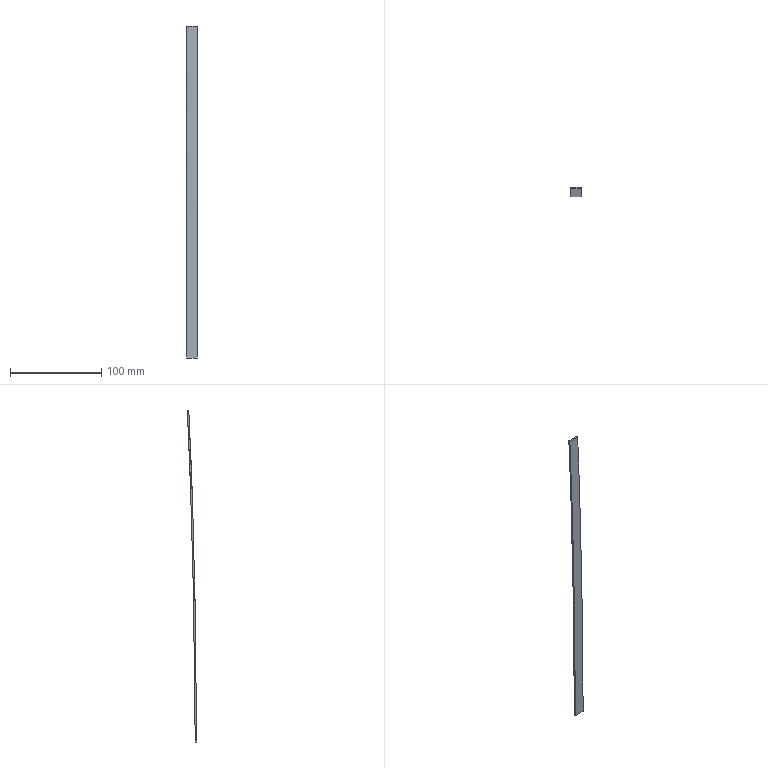Part | SolidWorks | features BaseBody 1 | 1 solid | 6 faces | box 12 x 10.218 x 364.25 mm | volume 6994 mm3 | plane 4 | spline 2
STEP:
#1=CARTESIAN_POINT('',(197.,-173.7,35.75));
#2=VERTEX_POINT('',#1);
#3=CARTESIAN_POINT('',(185.,-173.7,35.75));
#4=VERTEX_POINT('',#3);
#5=CARTESIAN_POINT('',(191.,-173.7,35.75));
#6=DIRECTION('',(-1.,0.,0.));
#7=VECTOR('',#6,1000.);
#8=LINE('',#5,#7);
#9=EDGE_CURVE('',#2,#4,#8,.T.);
#10=ORIENTED_EDGE('',*,*,#9,.T.);
#11=CARTESIAN_POINT('',(185.,-172.1,35.75));
#12=VERTEX_POINT('',#11);
#13=CARTESIAN_POINT('',(185.,-168.591,35.75));
#14=DIRECTION('',(0.,-1.,0.));
#15=VECTOR('',#14,1000.);
#16=LINE('',#13,#15);
#17=EDGE_CURVE('',#12,#4,#16,.T.);
#18=ORIENTED_EDGE('',*,*,#17,.F.);
#19=CARTESIAN_POINT('',(197.,-172.1,35.75));
#20=VERTEX_POINT('',#19);
#21=CARTESIAN_POINT('',(191.,-172.1,35.75));
#22=DIRECTION('',(1.,0.,0.));
#23=VECTOR('',#22,1000.);
#24=LINE('',#21,#23);
#25=EDGE_CURVE('',#12,#20,#24,.T.);
#26=ORIENTED_EDGE('',*,*,#25,.T.);
#27=CARTESIAN_POINT('',(197.,-168.591,35.75));
#28=DIRECTION('',(0.,1.,0.));
#29=VECTOR('',#28,1000.);
#30=LINE('',#27,#29);
#31=EDGE_CURVE('',#2,#20,#30,.T.);
#32=ORIENTED_EDGE('',*,*,#31,.F.);
#33=EDGE_LOOP('',(#10,#18,#26,#32));
#34=FACE_OUTER_BOUND('',#33,.T.);
#35=CARTESIAN_POINT('',(197.,-173.7,35.75));
#36=DIRECTION('',(0.,0.,-1.));
#37=DIRECTION('',(-1.,0.,0.));
#38=AXIS2_PLACEMENT_3D('',#35,#36,#37);
#39=PLANE('',#38);
#40=ADVANCED_FACE('',(#34),#39,.T.);
#41=ORIENTED_EDGE('',*,*,#9,.F.);
#42=CARTESIAN_POINT('',(197.,-165.082,400.));
#43=VERTEX_POINT('',#42);
#44=CARTESIAN_POINT('',(197.,-173.7,35.75));
#45=CARTESIAN_POINT('',(197.,-172.778,235.241));
#46=CARTESIAN_POINT('',(197.,-167.364,355.029));
#47=CARTESIAN_POINT('',(197.,-165.082,400.));
#48=B_SPLINE_CURVE_WITH_KNOTS('',3,(#44,#45,#46,#47),.UNSPECIFIED.,.F.,.F.,(4,4),(0.,0.3644),.UNSPECIFIED.);
#49=EDGE_CURVE('',#2,#43,#48,.T.);
#50=ORIENTED_EDGE('',*,*,#49,.T.);
#51=CARTESIAN_POINT('',(185.,-165.082,400.));
#52=VERTEX_POINT('',#51);
#53=CARTESIAN_POINT('',(190.94,-165.082,400.));
#54=DIRECTION('',(-1.,0.,0.));
#55=VECTOR('',#54,1000.);
#56=LINE('',#53,#55);
#57=EDGE_CURVE('',#43,#52,#56,.T.);
#58=ORIENTED_EDGE('',*,*,#57,.T.);
#59=CARTESIAN_POINT('',(185.,-165.082,400.));
#60=CARTESIAN_POINT('',(185.,-167.364,355.029));
#61=CARTESIAN_POINT('',(185.,-172.778,235.241));
#62=CARTESIAN_POINT('',(185.,-173.7,35.75));
#63=B_SPLINE_CURVE_WITH_KNOTS('',3,(#59,#60,#61,#62),.UNSPECIFIED.,.F.,.F.,(4,4),(0.,0.3644),.UNSPECIFIED.);
#64=EDGE_CURVE('',#52,#4,#63,.T.);
#65=ORIENTED_EDGE('',*,*,#64,.T.);
#66=EDGE_LOOP('',(#41,#50,#58,#65));
#67=FACE_OUTER_BOUND('',#66,.T.);
#68=CARTESIAN_POINT('',(197.,-165.082,400.));
#69=CARTESIAN_POINT('',(197.,-167.364,355.029));
#70=CARTESIAN_POINT('',(197.,-172.778,235.241));
#71=CARTESIAN_POINT('',(197.,-173.7,35.75));
#72=CARTESIAN_POINT('',(196.,-165.082,400.));
#73=CARTESIAN_POINT('',(196.,-167.364,355.029));
#74=CARTESIAN_POINT('',(196.,-172.778,235.241));
#75=CARTESIAN_POINT('',(196.,-173.7,35.75));
#76=CARTESIAN_POINT('',(194.,-165.082,400.));
#77=CARTESIAN_POINT('',(194.,-167.364,355.029));
#78=CARTESIAN_POINT('',(194.,-172.778,235.241));
#79=CARTESIAN_POINT('',(194.,-173.7,35.75));
#80=CARTESIAN_POINT('',(191.,-165.082,400.));
#81=CARTESIAN_POINT('',(191.,-167.364,355.029));
#82=CARTESIAN_POINT('',(191.,-172.778,235.241));
#83=CARTESIAN_POINT('',(191.,-173.7,35.75));
#84=CARTESIAN_POINT('',(188.,-165.082,400.));
#85=CARTESIAN_POINT('',(188.,-167.364,355.029));
#86=CARTESIAN_POINT('',(188.,-172.778,235.241));
#87=CARTESIAN_POINT('',(188.,-173.7,35.75));
#88=CARTESIAN_POINT('',(186.,-165.082,400.));
#89=CARTESIAN_POINT('',(186.,-167.364,355.029));
#90=CARTESIAN_POINT('',(186.,-172.778,235.241));
#91=CARTESIAN_POINT('',(186.,-173.7,35.75));
#92=CARTESIAN_POINT('',(185.,-165.082,400.));
#93=CARTESIAN_POINT('',(185.,-167.364,355.029));
#94=CARTESIAN_POINT('',(185.,-172.778,235.241));
#95=CARTESIAN_POINT('',(185.,-173.7,35.75));
#96=CARTESIAN_POINT('',(184.96,-165.082,400.));
#97=CARTESIAN_POINT('',(184.96,-167.364,355.029));
#98=CARTESIAN_POINT('',(184.96,-172.778,235.241));
#99=CARTESIAN_POINT('',(184.96,-173.7,35.75));
#100=CARTESIAN_POINT('',(184.92,-165.082,400.));
#101=CARTESIAN_POINT('',(184.92,-167.364,355.029));
#102=CARTESIAN_POINT('',(184.92,-172.778,235.241));
#103=CARTESIAN_POINT('',(184.92,-173.7,35.75));
#104=CARTESIAN_POINT('',(184.88,-165.082,400.));
#105=CARTESIAN_POINT('',(184.88,-167.364,355.029));
#106=CARTESIAN_POINT('',(184.88,-172.778,235.241));
#107=CARTESIAN_POINT('',(184.88,-173.7,35.75));
#108=B_SPLINE_SURFACE_WITH_KNOTS('',3,3,((#68,#69,#70,#71),(#72,#73,#74,#75),(#76,#77,#78,#79),(#80,#81,#82,#83),(#84,#85,#86,#87),(#88,#89,#90,#91),(#92,#93,#94,#95),(#96,#97,#98,#99),(#100,#101,#102,#103),(#104,#105,#106,#107)),.UNSPECIFIED.,.F.,.F.,.F.,(4,1,1,1,3,4),(4,4),(0.,0.1103,0.2206,0.3309,0.4412,0.4456),(0.,1.),.UNSPECIFIED.);
#109=ADVANCED_FACE('',(#67),#108,.T.);
#110=ORIENTED_EDGE('',*,*,#25,.F.);
#111=CARTESIAN_POINT('',(185.,-163.482,400.));
#112=VERTEX_POINT('',#111);
#113=CARTESIAN_POINT('',(185.,-172.1,35.75));
#114=CARTESIAN_POINT('',(185.,-171.178,235.241));
#115=CARTESIAN_POINT('',(185.,-165.764,355.029));
#116=CARTESIAN_POINT('',(185.,-163.482,400.));
#117=B_SPLINE_CURVE_WITH_KNOTS('',3,(#113,#114,#115,#116),.UNSPECIFIED.,.F.,.F.,(4,4),(0.,0.3644),.UNSPECIFIED.);
#118=EDGE_CURVE('',#12,#112,#117,.T.);
#119=ORIENTED_EDGE('',*,*,#118,.T.);
#120=CARTESIAN_POINT('',(197.,-163.482,400.));
#121=VERTEX_POINT('',#120);
#122=CARTESIAN_POINT('',(191.06,-163.482,400.));
#123=DIRECTION('',(1.,0.,0.));
#124=VECTOR('',#123,1000.);
#125=LINE('',#122,#124);
#126=EDGE_CURVE('',#112,#121,#125,.T.);
#127=ORIENTED_EDGE('',*,*,#126,.T.);
#128=CARTESIAN_POINT('',(197.,-163.482,400.));
#129=CARTESIAN_POINT('',(197.,-165.764,355.029));
#130=CARTESIAN_POINT('',(197.,-171.178,235.241));
#131=CARTESIAN_POINT('',(197.,-172.1,35.75));
#132=B_SPLINE_CURVE_WITH_KNOTS('',3,(#128,#129,#130,#131),.UNSPECIFIED.,.F.,.F.,(4,4),(0.,0.3644),.UNSPECIFIED.);
#133=EDGE_CURVE('',#121,#20,#132,.T.);
#134=ORIENTED_EDGE('',*,*,#133,.T.);
#135=EDGE_LOOP('',(#110,#119,#127,#134));
#136=FACE_OUTER_BOUND('',#135,.T.);
#137=CARTESIAN_POINT('',(185.,-163.482,400.));
#138=CARTESIAN_POINT('',(185.,-165.764,355.029));
#139=CARTESIAN_POINT('',(185.,-171.178,235.241));
#140=CARTESIAN_POINT('',(185.,-172.1,35.75));
#141=CARTESIAN_POINT('',(186.,-163.482,400.));
#142=CARTESIAN_POINT('',(186.,-165.764,355.029));
#143=CARTESIAN_POINT('',(186.,-171.178,235.241));
#144=CARTESIAN_POINT('',(186.,-172.1,35.75));
#145=CARTESIAN_POINT('',(188.,-163.482,400.));
#146=CARTESIAN_POINT('',(188.,-165.764,355.029));
#147=CARTESIAN_POINT('',(188.,-171.178,235.241));
#148=CARTESIAN_POINT('',(188.,-172.1,35.75));
#149=CARTESIAN_POINT('',(191.,-163.482,400.));
#150=CARTESIAN_POINT('',(191.,-165.764,355.029));
#151=CARTESIAN_POINT('',(191.,-171.178,235.241));
#152=CARTESIAN_POINT('',(191.,-172.1,35.75));
#153=CARTESIAN_POINT('',(194.,-163.482,400.));
#154=CARTESIAN_POINT('',(194.,-165.764,355.029));
#155=CARTESIAN_POINT('',(194.,-171.178,235.241));
#156=CARTESIAN_POINT('',(194.,-172.1,35.75));
#157=CARTESIAN_POINT('',(196.,-163.482,400.));
#158=CARTESIAN_POINT('',(196.,-165.764,355.029));
#159=CARTESIAN_POINT('',(196.,-171.178,235.241));
#160=CARTESIAN_POINT('',(196.,-172.1,35.75));
#161=CARTESIAN_POINT('',(197.,-163.482,400.));
#162=CARTESIAN_POINT('',(197.,-165.764,355.029));
#163=CARTESIAN_POINT('',(197.,-171.178,235.241));
#164=CARTESIAN_POINT('',(197.,-172.1,35.75));
#165=CARTESIAN_POINT('',(197.04,-163.482,400.));
#166=CARTESIAN_POINT('',(197.04,-165.764,355.029));
#167=CARTESIAN_POINT('',(197.04,-171.178,235.241));
#168=CARTESIAN_POINT('',(197.04,-172.1,35.75));
#169=CARTESIAN_POINT('',(197.08,-163.482,400.));
#170=CARTESIAN_POINT('',(197.08,-165.764,355.029));
#171=CARTESIAN_POINT('',(197.08,-171.178,235.241));
#172=CARTESIAN_POINT('',(197.08,-172.1,35.75));
#173=CARTESIAN_POINT('',(197.12,-163.482,400.));
#174=CARTESIAN_POINT('',(197.12,-165.764,355.029));
#175=CARTESIAN_POINT('',(197.12,-171.178,235.241));
#176=CARTESIAN_POINT('',(197.12,-172.1,35.75));
#177=B_SPLINE_SURFACE_WITH_KNOTS('',3,3,((#137,#138,#139,#140),(#141,#142,#143,#144),(#145,#146,#147,#148),(#149,#150,#151,#152),(#153,#154,#155,#156),(#157,#158,#159,#160),(#161,#162,#163,#164),(#165,#166,#167,#168),(#169,#170,#171,#172),(#173,#174,#175,#176)),.UNSPECIFIED.,.F.,.F.,.F.,(4,1,1,1,3,4),(4,4),(0.5,0.6103,0.7206,0.8309,0.9412,0.9456),(0.,1.),.UNSPECIFIED.);
#178=ADVANCED_FACE('',(#136),#177,.T.);
#179=ORIENTED_EDGE('',*,*,#31,.T.);
#180=ORIENTED_EDGE('',*,*,#133,.F.);
#181=CARTESIAN_POINT('',(197.,-168.591,400.));
#182=DIRECTION('',(0.,-1.,0.));
#183=VECTOR('',#182,1000.);
#184=LINE('',#181,#183);
#185=EDGE_CURVE('',#121,#43,#184,.T.);
#186=ORIENTED_EDGE('',*,*,#185,.T.);
#187=ORIENTED_EDGE('',*,*,#49,.F.);
#188=EDGE_LOOP('',(#179,#180,#186,#187));
#189=FACE_OUTER_BOUND('',#188,.T.);
#190=CARTESIAN_POINT('',(197.,-163.421,400.));
#191=DIRECTION('',(1.,0.,0.));
#192=DIRECTION('',(0.,-1.,0.));
#193=AXIS2_PLACEMENT_3D('',#190,#191,#192);
#194=PLANE('',#193);
#195=ADVANCED_FACE('',(#189),#194,.T.);
#196=ORIENTED_EDGE('',*,*,#17,.T.);
#197=ORIENTED_EDGE('',*,*,#64,.F.);
#198=CARTESIAN_POINT('',(185.,-168.591,400.));
#199=DIRECTION('',(0.,1.,0.));
#200=VECTOR('',#199,1000.);
#201=LINE('',#198,#200);
#202=EDGE_CURVE('',#52,#112,#201,.T.);
#203=ORIENTED_EDGE('',*,*,#202,.T.);
#204=ORIENTED_EDGE('',*,*,#118,.F.);
#205=EDGE_LOOP('',(#196,#197,#203,#204));
#206=FACE_OUTER_BOUND('',#205,.T.);
#207=CARTESIAN_POINT('',(185.,-173.761,400.));
#208=DIRECTION('',(-1.,0.,0.));
#209=DIRECTION('',(0.,1.,0.));
#210=AXIS2_PLACEMENT_3D('',#207,#208,#209);
#211=PLANE('',#210);
#212=ADVANCED_FACE('',(#206),#211,.T.);
#213=ORIENTED_EDGE('',*,*,#202,.F.);
#214=ORIENTED_EDGE('',*,*,#57,.F.);
#215=ORIENTED_EDGE('',*,*,#185,.F.);
#216=ORIENTED_EDGE('',*,*,#126,.F.);
#217=EDGE_LOOP('',(#213,#214,#215,#216));
#218=FACE_OUTER_BOUND('',#217,.T.);
#219=CARTESIAN_POINT('',(197.,-165.082,400.));
#220=DIRECTION('',(0.,0.,-1.));
#221=DIRECTION('',(-1.,0.,0.));
#222=AXIS2_PLACEMENT_3D('',#219,#220,#221);
#223=PLANE('',#222);
#224=ADVANCED_FACE('',(#218),#223,.F.);
#225=CLOSED_SHELL('',(#40,#109,#178,#195,#212,#224));
#226=MANIFOLD_SOLID_BREP('',#225);
#227=CARTESIAN_POINT('',(0.,0.,0.));
#228=DIRECTION('',(0.,0.,1.));
#229=DIRECTION('',(1.,0.,0.));
#230=AXIS2_PLACEMENT_3D('',#227,#228,#229);
#231=(LENGTH_UNIT()NAMED_UNIT(*)SI_UNIT(.MILLI.,.METRE.));
#232=UNCERTAINTY_MEASURE_WITH_UNIT(LENGTH_MEASURE(0.00001),#231,'','');
#233=(NAMED_UNIT(*)PLANE_ANGLE_UNIT()SI_UNIT($,.RADIAN.));
#234=(NAMED_UNIT(*)SI_UNIT($,.STERADIAN.)SOLID_ANGLE_UNIT());
#235=(GEOMETRIC_REPRESENTATION_CONTEXT(3)GLOBAL_UNCERTAINTY_ASSIGNED_CONTEXT((#232))GLOBAL_UNIT_ASSIGNED_CONTEXT((#231,#233,#234))REPRESENTATION_CONTEXT('',''));
#236=ADVANCED_BREP_SHAPE_REPRESENTATION('',(#226,#230),#235);